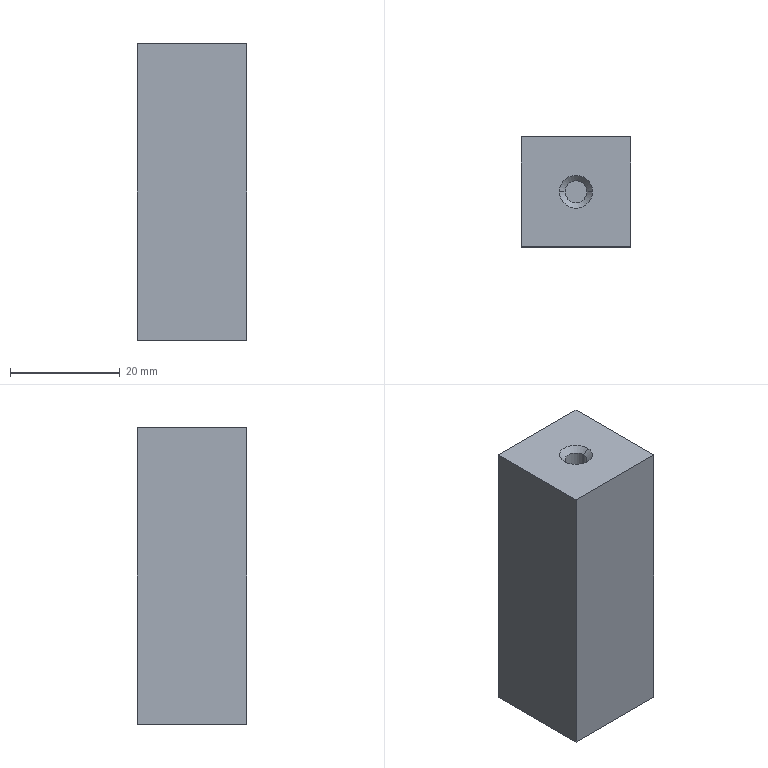Part | STEP file | Spacer block | 1 solid | 11 faces | box 20 x 20 x 54 mm | volume 21404 mm3 | plane 7 | cone 2 | cylinder 2 | commonest cylinder face diameters 4 x2
STEP:
#1=CARTESIAN_POINT('',(-10.868,-12.48,53.));
#2=VERTEX_POINT('',#1);
#3=CARTESIAN_POINT('',(-6.868,-12.48,53.));
#4=VERTEX_POINT('',#3);
#5=CARTESIAN_POINT('',(-8.868,-12.48,53.));
#6=DIRECTION('',(0.,0.,1.));
#7=DIRECTION('',(1.,0.,0.));
#8=AXIS2_PLACEMENT_3D('',#5,#6,#7);
#9=CIRCLE('',#8,2.);
#10=EDGE_CURVE('',#2,#4,#9,.T.);
#11=ORIENTED_EDGE('',*,*,#10,.F.);
#12=CARTESIAN_POINT('',(-11.868,-12.48,54.));
#13=VERTEX_POINT('',#12);
#14=CARTESIAN_POINT('',(-11.868,-12.48,54.));
#15=DIRECTION('',(-0.7071,0.,0.7071));
#16=VECTOR('',#15,1000.);
#17=LINE('',#14,#16);
#18=EDGE_CURVE('',#2,#13,#17,.T.);
#19=ORIENTED_EDGE('',*,*,#18,.T.);
#20=CARTESIAN_POINT('',(-5.868,-12.48,54.));
#21=VERTEX_POINT('',#20);
#22=CARTESIAN_POINT('',(-8.868,-12.48,54.));
#23=DIRECTION('',(0.,0.,-1.));
#24=DIRECTION('',(1.,0.,0.));
#25=AXIS2_PLACEMENT_3D('',#22,#23,#24);
#26=CIRCLE('',#25,3.);
#27=EDGE_CURVE('',#21,#13,#26,.T.);
#28=ORIENTED_EDGE('',*,*,#27,.F.);
#29=CARTESIAN_POINT('',(-5.868,-12.48,54.));
#30=DIRECTION('',(0.7071,0.,0.7071));
#31=VECTOR('',#30,1000.);
#32=LINE('',#29,#31);
#33=EDGE_CURVE('',#4,#21,#32,.T.);
#34=ORIENTED_EDGE('',*,*,#33,.F.);
#35=EDGE_LOOP('',(#11,#19,#28,#34));
#36=FACE_OUTER_BOUND('',#35,.T.);
#37=CARTESIAN_POINT('',(-8.868,-12.48,54.));
#38=DIRECTION('',(0.,0.,1.));
#39=DIRECTION('',(1.,0.,0.));
#40=AXIS2_PLACEMENT_3D('',#37,#38,#39);
#41=CONICAL_SURFACE('',#40,3.,0.7854);
#42=ADVANCED_FACE('',(#36),#41,.F.);
#43=CARTESIAN_POINT('',(-10.868,-12.48,39.));
#44=VERTEX_POINT('',#43);
#45=CARTESIAN_POINT('',(-6.868,-12.48,39.));
#46=VERTEX_POINT('',#45);
#47=CARTESIAN_POINT('',(-8.868,-12.48,39.));
#48=DIRECTION('',(0.,0.,1.));
#49=DIRECTION('',(1.,0.,0.));
#50=AXIS2_PLACEMENT_3D('',#47,#48,#49);
#51=CIRCLE('',#50,2.);
#52=EDGE_CURVE('',#44,#46,#51,.T.);
#53=ORIENTED_EDGE('',*,*,#52,.F.);
#54=CARTESIAN_POINT('',(-10.868,-12.48,39.));
#55=DIRECTION('',(0.,0.,1.));
#56=VECTOR('',#55,1000.);
#57=LINE('',#54,#56);
#58=EDGE_CURVE('',#44,#2,#57,.T.);
#59=ORIENTED_EDGE('',*,*,#58,.T.);
#60=ORIENTED_EDGE('',*,*,#10,.T.);
#61=CARTESIAN_POINT('',(-6.868,-12.48,39.));
#62=DIRECTION('',(0.,0.,1.));
#63=VECTOR('',#62,1000.);
#64=LINE('',#61,#63);
#65=EDGE_CURVE('',#46,#4,#64,.T.);
#66=ORIENTED_EDGE('',*,*,#65,.F.);
#67=EDGE_LOOP('',(#53,#59,#60,#66));
#68=FACE_OUTER_BOUND('',#67,.T.);
#69=CARTESIAN_POINT('',(-8.868,-12.48,39.));
#70=DIRECTION('',(0.,0.,1.));
#71=DIRECTION('',(1.,0.,0.));
#72=AXIS2_PLACEMENT_3D('',#69,#70,#71);
#73=CYLINDRICAL_SURFACE('',#72,2.);
#74=ADVANCED_FACE('',(#68),#73,.F.);
#75=CARTESIAN_POINT('',(-18.868,-22.48,54.));
#76=VERTEX_POINT('',#75);
#77=CARTESIAN_POINT('',(-18.868,-22.48,0.));
#78=VERTEX_POINT('',#77);
#79=CARTESIAN_POINT('',(-18.868,-22.48,54.));
#80=DIRECTION('',(0.,0.,-1.));
#81=VECTOR('',#80,1000.);
#82=LINE('',#79,#81);
#83=EDGE_CURVE('',#76,#78,#82,.T.);
#84=ORIENTED_EDGE('',*,*,#83,.F.);
#85=CARTESIAN_POINT('',(-18.868,-2.48,54.));
#86=VERTEX_POINT('',#85);
#87=CARTESIAN_POINT('',(-18.868,-2.48,54.));
#88=DIRECTION('',(0.,-1.,0.));
#89=VECTOR('',#88,1000.);
#90=LINE('',#87,#89);
#91=EDGE_CURVE('',#86,#76,#90,.T.);
#92=ORIENTED_EDGE('',*,*,#91,.F.);
#93=CARTESIAN_POINT('',(-18.868,-2.48,0.));
#94=VERTEX_POINT('',#93);
#95=CARTESIAN_POINT('',(-18.868,-2.48,54.));
#96=DIRECTION('',(0.,0.,1.));
#97=VECTOR('',#96,1000.);
#98=LINE('',#95,#97);
#99=EDGE_CURVE('',#94,#86,#98,.T.);
#100=ORIENTED_EDGE('',*,*,#99,.F.);
#101=CARTESIAN_POINT('',(-18.868,-2.48,0.));
#102=DIRECTION('',(0.,1.,0.));
#103=VECTOR('',#102,1000.);
#104=LINE('',#101,#103);
#105=EDGE_CURVE('',#78,#94,#104,.T.);
#106=ORIENTED_EDGE('',*,*,#105,.F.);
#107=EDGE_LOOP('',(#84,#92,#100,#106));
#108=FACE_OUTER_BOUND('',#107,.T.);
#109=CARTESIAN_POINT('',(-18.868,-2.48,54.));
#110=DIRECTION('',(1.,0.,0.));
#111=DIRECTION('',(0.,0.,-1.));
#112=AXIS2_PLACEMENT_3D('',#109,#110,#111);
#113=PLANE('',#112);
#114=ADVANCED_FACE('',(#108),#113,.F.);
#115=CARTESIAN_POINT('',(1.132,-2.48,0.));
#116=VERTEX_POINT('',#115);
#117=CARTESIAN_POINT('',(-18.868,-2.48,0.));
#118=DIRECTION('',(-1.,0.,0.));
#119=VECTOR('',#118,1000.);
#120=LINE('',#117,#119);
#121=EDGE_CURVE('',#116,#94,#120,.T.);
#122=ORIENTED_EDGE('',*,*,#121,.F.);
#123=CARTESIAN_POINT('',(1.132,-22.48,0.));
#124=VERTEX_POINT('',#123);
#125=CARTESIAN_POINT('',(1.132,-22.48,0.));
#126=DIRECTION('',(0.,1.,0.));
#127=VECTOR('',#126,1000.);
#128=LINE('',#125,#127);
#129=EDGE_CURVE('',#124,#116,#128,.T.);
#130=ORIENTED_EDGE('',*,*,#129,.F.);
#131=CARTESIAN_POINT('',(-18.868,-22.48,0.));
#132=DIRECTION('',(1.,0.,0.));
#133=VECTOR('',#132,1000.);
#134=LINE('',#131,#133);
#135=EDGE_CURVE('',#78,#124,#134,.T.);
#136=ORIENTED_EDGE('',*,*,#135,.F.);
#137=ORIENTED_EDGE('',*,*,#105,.T.);
#138=EDGE_LOOP('',(#122,#130,#136,#137));
#139=FACE_OUTER_BOUND('',#138,.T.);
#140=CARTESIAN_POINT('',(-18.868,-22.48,0.));
#141=DIRECTION('',(0.,0.,1.));
#142=DIRECTION('',(1.,0.,0.));
#143=AXIS2_PLACEMENT_3D('',#140,#141,#142);
#144=PLANE('',#143);
#145=ADVANCED_FACE('',(#139),#144,.F.);
#146=CARTESIAN_POINT('',(1.132,-22.48,54.));
#147=VERTEX_POINT('',#146);
#148=CARTESIAN_POINT('',(1.132,-22.48,54.));
#149=DIRECTION('',(0.,0.,-1.));
#150=VECTOR('',#149,1000.);
#151=LINE('',#148,#150);
#152=EDGE_CURVE('',#147,#124,#151,.T.);
#153=ORIENTED_EDGE('',*,*,#152,.F.);
#154=CARTESIAN_POINT('',(-18.868,-22.48,54.));
#155=DIRECTION('',(1.,0.,0.));
#156=VECTOR('',#155,1000.);
#157=LINE('',#154,#156);
#158=EDGE_CURVE('',#76,#147,#157,.T.);
#159=ORIENTED_EDGE('',*,*,#158,.F.);
#160=ORIENTED_EDGE('',*,*,#83,.T.);
#161=ORIENTED_EDGE('',*,*,#135,.T.);
#162=EDGE_LOOP('',(#153,#159,#160,#161));
#163=FACE_OUTER_BOUND('',#162,.T.);
#164=CARTESIAN_POINT('',(-18.868,-22.48,54.));
#165=DIRECTION('',(0.,1.,0.));
#166=DIRECTION('',(0.,0.,1.));
#167=AXIS2_PLACEMENT_3D('',#164,#165,#166);
#168=PLANE('',#167);
#169=ADVANCED_FACE('',(#163),#168,.F.);
#170=CARTESIAN_POINT('',(1.132,-2.48,54.));
#171=VERTEX_POINT('',#170);
#172=CARTESIAN_POINT('',(1.132,-22.48,54.));
#173=DIRECTION('',(0.,1.,0.));
#174=VECTOR('',#173,1000.);
#175=LINE('',#172,#174);
#176=EDGE_CURVE('',#147,#171,#175,.T.);
#177=ORIENTED_EDGE('',*,*,#176,.T.);
#178=CARTESIAN_POINT('',(-18.868,-2.48,54.));
#179=DIRECTION('',(-1.,0.,0.));
#180=VECTOR('',#179,1000.);
#181=LINE('',#178,#180);
#182=EDGE_CURVE('',#171,#86,#181,.T.);
#183=ORIENTED_EDGE('',*,*,#182,.T.);
#184=ORIENTED_EDGE('',*,*,#91,.T.);
#185=ORIENTED_EDGE('',*,*,#158,.T.);
#186=EDGE_LOOP('',(#177,#183,#184,#185));
#187=FACE_OUTER_BOUND('',#186,.T.);
#188=ORIENTED_EDGE('',*,*,#27,.T.);
#189=CARTESIAN_POINT('',(-8.868,-12.48,54.));
#190=DIRECTION('',(0.,0.,-1.));
#191=DIRECTION('',(1.,0.,0.));
#192=AXIS2_PLACEMENT_3D('',#189,#190,#191);
#193=CIRCLE('',#192,3.);
#194=EDGE_CURVE('',#13,#21,#193,.T.);
#195=ORIENTED_EDGE('',*,*,#194,.T.);
#196=EDGE_LOOP('',(#188,#195));
#197=FACE_BOUND('',#196,.T.);
#198=CARTESIAN_POINT('',(-18.868,-22.48,54.));
#199=DIRECTION('',(0.,0.,1.));
#200=DIRECTION('',(1.,0.,0.));
#201=AXIS2_PLACEMENT_3D('',#198,#199,#200);
#202=PLANE('',#201);
#203=ADVANCED_FACE('',(#187,#197),#202,.T.);
#204=ORIENTED_EDGE('',*,*,#99,.T.);
#205=ORIENTED_EDGE('',*,*,#182,.F.);
#206=CARTESIAN_POINT('',(1.132,-2.48,54.));
#207=DIRECTION('',(0.,0.,1.));
#208=VECTOR('',#207,1000.);
#209=LINE('',#206,#208);
#210=EDGE_CURVE('',#116,#171,#209,.T.);
#211=ORIENTED_EDGE('',*,*,#210,.F.);
#212=ORIENTED_EDGE('',*,*,#121,.T.);
#213=EDGE_LOOP('',(#204,#205,#211,#212));
#214=FACE_OUTER_BOUND('',#213,.T.);
#215=CARTESIAN_POINT('',(-18.868,-2.48,54.));
#216=DIRECTION('',(0.,-1.,0.));
#217=DIRECTION('',(0.,0.,-1.));
#218=AXIS2_PLACEMENT_3D('',#215,#216,#217);
#219=PLANE('',#218);
#220=ADVANCED_FACE('',(#214),#219,.F.);
#221=ORIENTED_EDGE('',*,*,#210,.T.);
#222=ORIENTED_EDGE('',*,*,#176,.F.);
#223=ORIENTED_EDGE('',*,*,#152,.T.);
#224=ORIENTED_EDGE('',*,*,#129,.T.);
#225=EDGE_LOOP('',(#221,#222,#223,#224));
#226=FACE_OUTER_BOUND('',#225,.T.);
#227=CARTESIAN_POINT('',(1.132,-2.48,54.));
#228=DIRECTION('',(-1.,0.,0.));
#229=DIRECTION('',(0.,0.,1.));
#230=AXIS2_PLACEMENT_3D('',#227,#228,#229);
#231=PLANE('',#230);
#232=ADVANCED_FACE('',(#226),#231,.F.);
#233=ORIENTED_EDGE('',*,*,#18,.F.);
#234=CARTESIAN_POINT('',(-8.868,-12.48,53.));
#235=DIRECTION('',(0.,0.,1.));
#236=DIRECTION('',(1.,0.,0.));
#237=AXIS2_PLACEMENT_3D('',#234,#235,#236);
#238=CIRCLE('',#237,2.);
#239=EDGE_CURVE('',#4,#2,#238,.T.);
#240=ORIENTED_EDGE('',*,*,#239,.F.);
#241=ORIENTED_EDGE('',*,*,#33,.T.);
#242=ORIENTED_EDGE('',*,*,#194,.F.);
#243=EDGE_LOOP('',(#233,#240,#241,#242));
#244=FACE_OUTER_BOUND('',#243,.T.);
#245=CARTESIAN_POINT('',(-8.868,-12.48,54.));
#246=DIRECTION('',(0.,0.,1.));
#247=DIRECTION('',(1.,0.,0.));
#248=AXIS2_PLACEMENT_3D('',#245,#246,#247);
#249=CONICAL_SURFACE('',#248,3.,0.7854);
#250=ADVANCED_FACE('',(#244),#249,.F.);
#251=ORIENTED_EDGE('',*,*,#58,.F.);
#252=CARTESIAN_POINT('',(-8.868,-12.48,39.));
#253=DIRECTION('',(0.,0.,1.));
#254=DIRECTION('',(1.,0.,0.));
#255=AXIS2_PLACEMENT_3D('',#252,#253,#254);
#256=CIRCLE('',#255,2.);
#257=EDGE_CURVE('',#46,#44,#256,.T.);
#258=ORIENTED_EDGE('',*,*,#257,.F.);
#259=ORIENTED_EDGE('',*,*,#65,.T.);
#260=ORIENTED_EDGE('',*,*,#239,.T.);
#261=EDGE_LOOP('',(#251,#258,#259,#260));
#262=FACE_OUTER_BOUND('',#261,.T.);
#263=CARTESIAN_POINT('',(-8.868,-12.48,39.));
#264=DIRECTION('',(0.,0.,1.));
#265=DIRECTION('',(1.,0.,0.));
#266=AXIS2_PLACEMENT_3D('',#263,#264,#265);
#267=CYLINDRICAL_SURFACE('',#266,2.);
#268=ADVANCED_FACE('',(#262),#267,.F.);
#269=ORIENTED_EDGE('',*,*,#257,.T.);
#270=ORIENTED_EDGE('',*,*,#52,.T.);
#271=EDGE_LOOP('',(#269,#270));
#272=FACE_OUTER_BOUND('',#271,.T.);
#273=CARTESIAN_POINT('',(-8.868,-12.48,39.));
#274=DIRECTION('',(0.,0.,1.));
#275=DIRECTION('',(1.,0.,0.));
#276=AXIS2_PLACEMENT_3D('',#273,#274,#275);
#277=PLANE('',#276);
#278=ADVANCED_FACE('',(#272),#277,.T.);
#279=CLOSED_SHELL('',(#42,#74,#114,#145,#169,#203,#220,#232,#250,#268,#278));
#280=MANIFOLD_SOLID_BREP('',#279);
#281=CARTESIAN_POINT('',(0.,0.,0.));
#282=DIRECTION('',(0.,0.,1.));
#283=DIRECTION('',(1.,0.,0.));
#284=AXIS2_PLACEMENT_3D('',#281,#282,#283);
#285=(LENGTH_UNIT()NAMED_UNIT(*)SI_UNIT(.MILLI.,.METRE.));
#286=UNCERTAINTY_MEASURE_WITH_UNIT(LENGTH_MEASURE(0.00001),#285,'','');
#287=(NAMED_UNIT(*)PLANE_ANGLE_UNIT()SI_UNIT($,.RADIAN.));
#288=(NAMED_UNIT(*)SI_UNIT($,.STERADIAN.)SOLID_ANGLE_UNIT());
#289=(GEOMETRIC_REPRESENTATION_CONTEXT(3)GLOBAL_UNCERTAINTY_ASSIGNED_CONTEXT((#286))GLOBAL_UNIT_ASSIGNED_CONTEXT((#285,#287,#288))REPRESENTATION_CONTEXT('',''));
#290=ADVANCED_BREP_SHAPE_REPRESENTATION('',(#280,#284),#289);